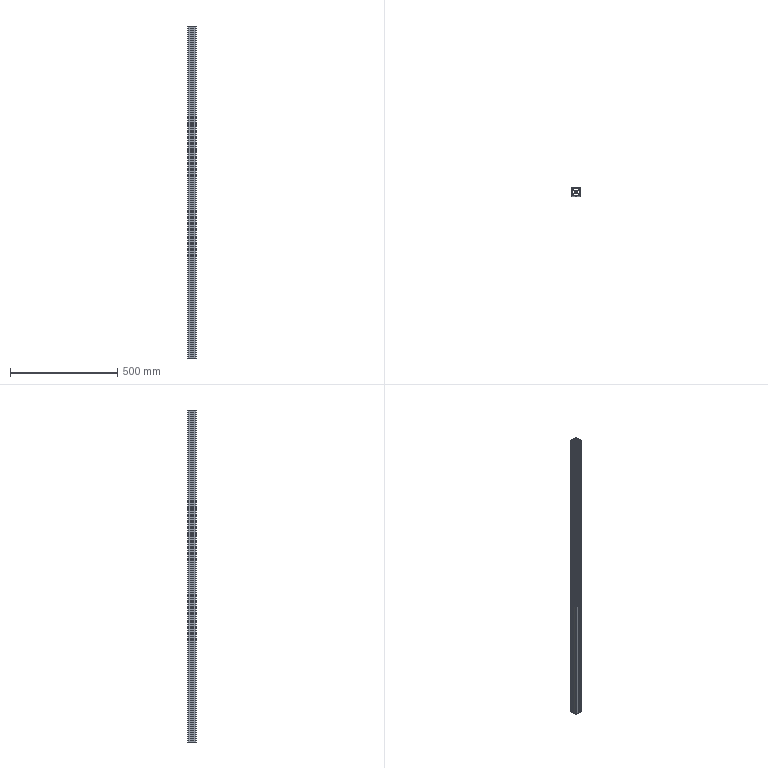Part | SolidWorks | features Extrusion 1 | 1 solid | 147 faces | box 40 x 40 x 1548 mm | volume 930498 mm3 | plane 117 | cylinder 30 | commonest cylinder face diameters 1 x8 2 x8 6.8 x5 5 x4 9 x4 1.414 x1